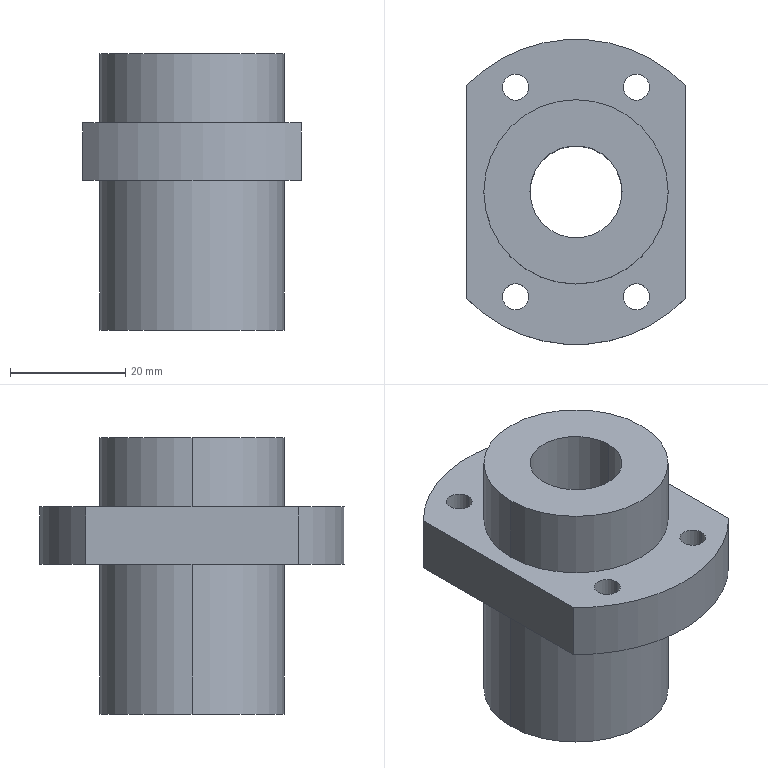Part | STEP file | Ball screw 4R16-16S2-DFSH-920-982-0.05(S)_HIWEI_default | 1 solid | 22 faces | box 38 x 53 x 48 mm | volume 38522 mm3 | cylinder 16 | plane 6 | commonest cylinder face diameters 4.5 x8 32 x4 16 x2 53 x2
STEP:
#1=CARTESIAN_POINT('',(-16.,0.,26.));
#2=VERTEX_POINT('',#1);
#3=CARTESIAN_POINT('',(16.,0.,26.));
#4=VERTEX_POINT('',#3);
#5=CARTESIAN_POINT('',(0.,0.,26.));
#6=DIRECTION('',(0.,0.,-1.));
#7=DIRECTION('',(-1.,0.,0.));
#8=AXIS2_PLACEMENT_3D('',#5,#6,#7);
#9=CIRCLE('',#8,16.);
#10=EDGE_CURVE('',#2,#4,#9,.T.);
#11=ORIENTED_EDGE('',*,*,#10,.T.);
#12=CARTESIAN_POINT('',(16.,0.,0.));
#13=VERTEX_POINT('',#12);
#14=CARTESIAN_POINT('',(16.,0.,48.));
#15=DIRECTION('',(0.,0.,-1.));
#16=VECTOR('',#15,1000.);
#17=LINE('',#14,#16);
#18=EDGE_CURVE('',#4,#13,#17,.T.);
#19=ORIENTED_EDGE('',*,*,#18,.T.);
#20=CARTESIAN_POINT('',(-16.,0.,0.));
#21=VERTEX_POINT('',#20);
#22=CARTESIAN_POINT('',(0.,0.,0.));
#23=DIRECTION('',(0.,0.,1.));
#24=DIRECTION('',(-1.,0.,0.));
#25=AXIS2_PLACEMENT_3D('',#22,#23,#24);
#26=CIRCLE('',#25,16.);
#27=EDGE_CURVE('',#13,#21,#26,.T.);
#28=ORIENTED_EDGE('',*,*,#27,.T.);
#29=CARTESIAN_POINT('',(-16.,0.,48.));
#30=DIRECTION('',(0.,0.,-1.));
#31=VECTOR('',#30,1000.);
#32=LINE('',#29,#31);
#33=EDGE_CURVE('',#2,#21,#32,.T.);
#34=ORIENTED_EDGE('',*,*,#33,.F.);
#35=EDGE_LOOP('',(#11,#19,#28,#34));
#36=FACE_OUTER_BOUND('',#35,.T.);
#37=CARTESIAN_POINT('',(0.,0.,48.));
#38=DIRECTION('',(0.,0.,-1.));
#39=DIRECTION('',(-1.,0.,0.));
#40=AXIS2_PLACEMENT_3D('',#37,#38,#39);
#41=CYLINDRICAL_SURFACE('',#40,16.);
#42=ADVANCED_FACE('',(#36),#41,.T.);
#43=CARTESIAN_POINT('',(8.,0.,48.));
#44=VERTEX_POINT('',#43);
#45=CARTESIAN_POINT('',(-8.,0.,48.));
#46=VERTEX_POINT('',#45);
#47=CARTESIAN_POINT('',(0.,0.,48.));
#48=DIRECTION('',(0.,0.,-1.));
#49=DIRECTION('',(-1.,0.,0.));
#50=AXIS2_PLACEMENT_3D('',#47,#48,#49);
#51=CIRCLE('',#50,8.);
#52=EDGE_CURVE('',#44,#46,#51,.T.);
#53=ORIENTED_EDGE('',*,*,#52,.F.);
#54=CARTESIAN_POINT('',(8.,0.,0.));
#55=VERTEX_POINT('',#54);
#56=CARTESIAN_POINT('',(8.,0.,160.));
#57=DIRECTION('',(0.,0.,-1.));
#58=VECTOR('',#57,1000.);
#59=LINE('',#56,#58);
#60=EDGE_CURVE('',#44,#55,#59,.T.);
#61=ORIENTED_EDGE('',*,*,#60,.T.);
#62=CARTESIAN_POINT('',(-8.,0.,0.));
#63=VERTEX_POINT('',#62);
#64=CARTESIAN_POINT('',(0.,0.,0.));
#65=DIRECTION('',(0.,0.,-1.));
#66=DIRECTION('',(-1.,0.,0.));
#67=AXIS2_PLACEMENT_3D('',#64,#65,#66);
#68=CIRCLE('',#67,8.);
#69=EDGE_CURVE('',#55,#63,#68,.T.);
#70=ORIENTED_EDGE('',*,*,#69,.T.);
#71=CARTESIAN_POINT('',(-8.,0.,160.));
#72=DIRECTION('',(0.,0.,-1.));
#73=VECTOR('',#72,1000.);
#74=LINE('',#71,#73);
#75=EDGE_CURVE('',#46,#63,#74,.T.);
#76=ORIENTED_EDGE('',*,*,#75,.F.);
#77=EDGE_LOOP('',(#53,#61,#70,#76));
#78=FACE_OUTER_BOUND('',#77,.T.);
#79=CARTESIAN_POINT('',(0.,0.,160.));
#80=DIRECTION('',(0.,0.,-1.));
#81=DIRECTION('',(-1.,0.,0.));
#82=AXIS2_PLACEMENT_3D('',#79,#80,#81);
#83=CYLINDRICAL_SURFACE('',#82,8.);
#84=ADVANCED_FACE('',(#78),#83,.F.);
#85=CARTESIAN_POINT('',(12.75,-18.187,26.));
#86=VERTEX_POINT('',#85);
#87=CARTESIAN_POINT('',(8.25,-18.187,26.));
#88=VERTEX_POINT('',#87);
#89=CARTESIAN_POINT('',(10.5,-18.187,26.));
#90=DIRECTION('',(0.,0.,-1.));
#91=DIRECTION('',(1.,0.,0.));
#92=AXIS2_PLACEMENT_3D('',#89,#90,#91);
#93=CIRCLE('',#92,2.25);
#94=EDGE_CURVE('',#86,#88,#93,.T.);
#95=ORIENTED_EDGE('',*,*,#94,.T.);
#96=CARTESIAN_POINT('',(8.25,-18.187,36.));
#97=VERTEX_POINT('',#96);
#98=CARTESIAN_POINT('',(8.25,-18.187,26.));
#99=DIRECTION('',(0.,0.,1.));
#100=VECTOR('',#99,1000.);
#101=LINE('',#98,#100);
#102=EDGE_CURVE('',#88,#97,#101,.T.);
#103=ORIENTED_EDGE('',*,*,#102,.T.);
#104=CARTESIAN_POINT('',(12.75,-18.187,36.));
#105=VERTEX_POINT('',#104);
#106=CARTESIAN_POINT('',(10.5,-18.187,36.));
#107=DIRECTION('',(0.,0.,-1.));
#108=DIRECTION('',(1.,0.,0.));
#109=AXIS2_PLACEMENT_3D('',#106,#107,#108);
#110=CIRCLE('',#109,2.25);
#111=EDGE_CURVE('',#105,#97,#110,.T.);
#112=ORIENTED_EDGE('',*,*,#111,.F.);
#113=CARTESIAN_POINT('',(12.75,-18.187,26.));
#114=DIRECTION('',(0.,0.,1.));
#115=VECTOR('',#114,1000.);
#116=LINE('',#113,#115);
#117=EDGE_CURVE('',#86,#105,#116,.T.);
#118=ORIENTED_EDGE('',*,*,#117,.F.);
#119=EDGE_LOOP('',(#95,#103,#112,#118));
#120=FACE_OUTER_BOUND('',#119,.T.);
#121=CARTESIAN_POINT('',(10.5,-18.187,26.));
#122=DIRECTION('',(0.,0.,1.));
#123=DIRECTION('',(1.,0.,0.));
#124=AXIS2_PLACEMENT_3D('',#121,#122,#123);
#125=CYLINDRICAL_SURFACE('',#124,2.25);
#126=ADVANCED_FACE('',(#120),#125,.F.);
#127=CARTESIAN_POINT('',(-8.25,18.187,26.));
#128=VERTEX_POINT('',#127);
#129=CARTESIAN_POINT('',(-12.75,18.187,26.));
#130=VERTEX_POINT('',#129);
#131=CARTESIAN_POINT('',(-10.5,18.187,26.));
#132=DIRECTION('',(0.,0.,-1.));
#133=DIRECTION('',(1.,0.,0.));
#134=AXIS2_PLACEMENT_3D('',#131,#132,#133);
#135=CIRCLE('',#134,2.25);
#136=EDGE_CURVE('',#128,#130,#135,.T.);
#137=ORIENTED_EDGE('',*,*,#136,.T.);
#138=CARTESIAN_POINT('',(-12.75,18.187,36.));
#139=VERTEX_POINT('',#138);
#140=CARTESIAN_POINT('',(-12.75,18.187,26.));
#141=DIRECTION('',(0.,0.,1.));
#142=VECTOR('',#141,1000.);
#143=LINE('',#140,#142);
#144=EDGE_CURVE('',#130,#139,#143,.T.);
#145=ORIENTED_EDGE('',*,*,#144,.T.);
#146=CARTESIAN_POINT('',(-8.25,18.187,36.));
#147=VERTEX_POINT('',#146);
#148=CARTESIAN_POINT('',(-10.5,18.187,36.));
#149=DIRECTION('',(0.,0.,-1.));
#150=DIRECTION('',(1.,0.,0.));
#151=AXIS2_PLACEMENT_3D('',#148,#149,#150);
#152=CIRCLE('',#151,2.25);
#153=EDGE_CURVE('',#147,#139,#152,.T.);
#154=ORIENTED_EDGE('',*,*,#153,.F.);
#155=CARTESIAN_POINT('',(-8.25,18.187,26.));
#156=DIRECTION('',(0.,0.,1.));
#157=VECTOR('',#156,1000.);
#158=LINE('',#155,#157);
#159=EDGE_CURVE('',#128,#147,#158,.T.);
#160=ORIENTED_EDGE('',*,*,#159,.F.);
#161=EDGE_LOOP('',(#137,#145,#154,#160));
#162=FACE_OUTER_BOUND('',#161,.T.);
#163=CARTESIAN_POINT('',(-10.5,18.187,26.));
#164=DIRECTION('',(0.,0.,1.));
#165=DIRECTION('',(1.,0.,0.));
#166=AXIS2_PLACEMENT_3D('',#163,#164,#165);
#167=CYLINDRICAL_SURFACE('',#166,2.25);
#168=ADVANCED_FACE('',(#162),#167,.F.);
#169=CARTESIAN_POINT('',(12.75,18.187,26.));
#170=VERTEX_POINT('',#169);
#171=CARTESIAN_POINT('',(8.25,18.187,26.));
#172=VERTEX_POINT('',#171);
#173=CARTESIAN_POINT('',(10.5,18.187,26.));
#174=DIRECTION('',(0.,0.,-1.));
#175=DIRECTION('',(1.,0.,0.));
#176=AXIS2_PLACEMENT_3D('',#173,#174,#175);
#177=CIRCLE('',#176,2.25);
#178=EDGE_CURVE('',#170,#172,#177,.T.);
#179=ORIENTED_EDGE('',*,*,#178,.T.);
#180=CARTESIAN_POINT('',(8.25,18.187,36.));
#181=VERTEX_POINT('',#180);
#182=CARTESIAN_POINT('',(8.25,18.187,26.));
#183=DIRECTION('',(0.,0.,1.));
#184=VECTOR('',#183,1000.);
#185=LINE('',#182,#184);
#186=EDGE_CURVE('',#172,#181,#185,.T.);
#187=ORIENTED_EDGE('',*,*,#186,.T.);
#188=CARTESIAN_POINT('',(12.75,18.187,36.));
#189=VERTEX_POINT('',#188);
#190=CARTESIAN_POINT('',(10.5,18.187,36.));
#191=DIRECTION('',(0.,0.,-1.));
#192=DIRECTION('',(1.,0.,0.));
#193=AXIS2_PLACEMENT_3D('',#190,#191,#192);
#194=CIRCLE('',#193,2.25);
#195=EDGE_CURVE('',#189,#181,#194,.T.);
#196=ORIENTED_EDGE('',*,*,#195,.F.);
#197=CARTESIAN_POINT('',(12.75,18.187,26.));
#198=DIRECTION('',(0.,0.,1.));
#199=VECTOR('',#198,1000.);
#200=LINE('',#197,#199);
#201=EDGE_CURVE('',#170,#189,#200,.T.);
#202=ORIENTED_EDGE('',*,*,#201,.F.);
#203=EDGE_LOOP('',(#179,#187,#196,#202));
#204=FACE_OUTER_BOUND('',#203,.T.);
#205=CARTESIAN_POINT('',(10.5,18.187,26.));
#206=DIRECTION('',(0.,0.,1.));
#207=DIRECTION('',(1.,0.,0.));
#208=AXIS2_PLACEMENT_3D('',#205,#206,#207);
#209=CYLINDRICAL_SURFACE('',#208,2.25);
#210=ADVANCED_FACE('',(#204),#209,.F.);
#211=CARTESIAN_POINT('',(-8.25,-18.187,26.));
#212=VERTEX_POINT('',#211);
#213=CARTESIAN_POINT('',(-12.75,-18.187,26.));
#214=VERTEX_POINT('',#213);
#215=CARTESIAN_POINT('',(-10.5,-18.187,26.));
#216=DIRECTION('',(0.,0.,-1.));
#217=DIRECTION('',(1.,0.,0.));
#218=AXIS2_PLACEMENT_3D('',#215,#216,#217);
#219=CIRCLE('',#218,2.25);
#220=EDGE_CURVE('',#212,#214,#219,.T.);
#221=ORIENTED_EDGE('',*,*,#220,.T.);
#222=CARTESIAN_POINT('',(-12.75,-18.187,36.));
#223=VERTEX_POINT('',#222);
#224=CARTESIAN_POINT('',(-12.75,-18.187,26.));
#225=DIRECTION('',(0.,0.,1.));
#226=VECTOR('',#225,1000.);
#227=LINE('',#224,#226);
#228=EDGE_CURVE('',#214,#223,#227,.T.);
#229=ORIENTED_EDGE('',*,*,#228,.T.);
#230=CARTESIAN_POINT('',(-8.25,-18.187,36.));
#231=VERTEX_POINT('',#230);
#232=CARTESIAN_POINT('',(-10.5,-18.187,36.));
#233=DIRECTION('',(0.,0.,-1.));
#234=DIRECTION('',(1.,0.,0.));
#235=AXIS2_PLACEMENT_3D('',#232,#233,#234);
#236=CIRCLE('',#235,2.25);
#237=EDGE_CURVE('',#231,#223,#236,.T.);
#238=ORIENTED_EDGE('',*,*,#237,.F.);
#239=CARTESIAN_POINT('',(-8.25,-18.187,26.));
#240=DIRECTION('',(0.,0.,1.));
#241=VECTOR('',#240,1000.);
#242=LINE('',#239,#241);
#243=EDGE_CURVE('',#212,#231,#242,.T.);
#244=ORIENTED_EDGE('',*,*,#243,.F.);
#245=EDGE_LOOP('',(#221,#229,#238,#244));
#246=FACE_OUTER_BOUND('',#245,.T.);
#247=CARTESIAN_POINT('',(-10.5,-18.187,26.));
#248=DIRECTION('',(0.,0.,1.));
#249=DIRECTION('',(1.,0.,0.));
#250=AXIS2_PLACEMENT_3D('',#247,#248,#249);
#251=CYLINDRICAL_SURFACE('',#250,2.25);
#252=ADVANCED_FACE('',(#246),#251,.F.);
#253=CARTESIAN_POINT('',(16.,0.,48.));
#254=VERTEX_POINT('',#253);
#255=CARTESIAN_POINT('',(-16.,0.,48.));
#256=VERTEX_POINT('',#255);
#257=CARTESIAN_POINT('',(0.,0.,48.));
#258=DIRECTION('',(0.,0.,1.));
#259=DIRECTION('',(-1.,0.,0.));
#260=AXIS2_PLACEMENT_3D('',#257,#258,#259);
#261=CIRCLE('',#260,16.);
#262=EDGE_CURVE('',#254,#256,#261,.T.);
#263=ORIENTED_EDGE('',*,*,#262,.F.);
#264=CARTESIAN_POINT('',(16.,0.,36.));
#265=VERTEX_POINT('',#264);
#266=CARTESIAN_POINT('',(16.,0.,48.));
#267=DIRECTION('',(0.,0.,-1.));
#268=VECTOR('',#267,1000.);
#269=LINE('',#266,#268);
#270=EDGE_CURVE('',#254,#265,#269,.T.);
#271=ORIENTED_EDGE('',*,*,#270,.T.);
#272=CARTESIAN_POINT('',(-16.,0.,36.));
#273=VERTEX_POINT('',#272);
#274=CARTESIAN_POINT('',(0.,0.,36.));
#275=DIRECTION('',(0.,0.,-1.));
#276=DIRECTION('',(-1.,0.,0.));
#277=AXIS2_PLACEMENT_3D('',#274,#275,#276);
#278=CIRCLE('',#277,16.);
#279=EDGE_CURVE('',#273,#265,#278,.T.);
#280=ORIENTED_EDGE('',*,*,#279,.F.);
#281=CARTESIAN_POINT('',(-16.,0.,48.));
#282=DIRECTION('',(0.,0.,-1.));
#283=VECTOR('',#282,1000.);
#284=LINE('',#281,#283);
#285=EDGE_CURVE('',#256,#273,#284,.T.);
#286=ORIENTED_EDGE('',*,*,#285,.F.);
#287=EDGE_LOOP('',(#263,#271,#280,#286));
#288=FACE_OUTER_BOUND('',#287,.T.);
#289=CARTESIAN_POINT('',(0.,0.,48.));
#290=DIRECTION('',(0.,0.,-1.));
#291=DIRECTION('',(-1.,0.,0.));
#292=AXIS2_PLACEMENT_3D('',#289,#290,#291);
#293=CYLINDRICAL_SURFACE('',#292,16.);
#294=ADVANCED_FACE('',(#288),#293,.T.);
#295=ORIENTED_EDGE('',*,*,#18,.F.);
#296=CARTESIAN_POINT('',(0.,0.,26.));
#297=DIRECTION('',(0.,0.,-1.));
#298=DIRECTION('',(-1.,0.,0.));
#299=AXIS2_PLACEMENT_3D('',#296,#297,#298);
#300=CIRCLE('',#299,16.);
#301=EDGE_CURVE('',#4,#2,#300,.T.);
#302=ORIENTED_EDGE('',*,*,#301,.T.);
#303=ORIENTED_EDGE('',*,*,#33,.T.);
#304=CARTESIAN_POINT('',(0.,0.,0.));
#305=DIRECTION('',(0.,0.,1.));
#306=DIRECTION('',(-1.,0.,0.));
#307=AXIS2_PLACEMENT_3D('',#304,#305,#306);
#308=CIRCLE('',#307,16.);
#309=EDGE_CURVE('',#21,#13,#308,.T.);
#310=ORIENTED_EDGE('',*,*,#309,.T.);
#311=EDGE_LOOP('',(#295,#302,#303,#310));
#312=FACE_OUTER_BOUND('',#311,.T.);
#313=CARTESIAN_POINT('',(0.,0.,48.));
#314=DIRECTION('',(0.,0.,-1.));
#315=DIRECTION('',(-1.,0.,0.));
#316=AXIS2_PLACEMENT_3D('',#313,#314,#315);
#317=CYLINDRICAL_SURFACE('',#316,16.);
#318=ADVANCED_FACE('',(#312),#317,.T.);
#319=ORIENTED_EDGE('',*,*,#309,.F.);
#320=ORIENTED_EDGE('',*,*,#27,.F.);
#321=EDGE_LOOP('',(#319,#320));
#322=FACE_OUTER_BOUND('',#321,.T.);
#323=CARTESIAN_POINT('',(0.,0.,0.));
#324=DIRECTION('',(0.,0.,-1.));
#325=DIRECTION('',(-1.,0.,0.));
#326=AXIS2_PLACEMENT_3D('',#323,#324,#325);
#327=CIRCLE('',#326,8.);
#328=EDGE_CURVE('',#63,#55,#327,.T.);
#329=ORIENTED_EDGE('',*,*,#328,.F.);
#330=ORIENTED_EDGE('',*,*,#69,.F.);
#331=EDGE_LOOP('',(#329,#330));
#332=FACE_BOUND('',#331,.T.);
#333=CARTESIAN_POINT('',(0.,0.,0.));
#334=DIRECTION('',(0.,0.,1.));
#335=DIRECTION('',(1.,0.,0.));
#336=AXIS2_PLACEMENT_3D('',#333,#334,#335);
#337=PLANE('',#336);
#338=ADVANCED_FACE('',(#322,#332),#337,.F.);
#339=ORIENTED_EDGE('',*,*,#94,.F.);
#340=CARTESIAN_POINT('',(10.5,-18.187,26.));
#341=DIRECTION('',(0.,0.,-1.));
#342=DIRECTION('',(1.,0.,0.));
#343=AXIS2_PLACEMENT_3D('',#340,#341,#342);
#344=CIRCLE('',#343,2.25);
#345=EDGE_CURVE('',#88,#86,#344,.T.);
#346=ORIENTED_EDGE('',*,*,#345,.F.);
#347=EDGE_LOOP('',(#339,#346));
#348=FACE_BOUND('',#347,.T.);
#349=ORIENTED_EDGE('',*,*,#10,.F.);
#350=ORIENTED_EDGE('',*,*,#301,.F.);
#351=EDGE_LOOP('',(#349,#350));
#352=FACE_BOUND('',#351,.T.);
#353=CARTESIAN_POINT('',(19.,-18.473,26.));
#354=VERTEX_POINT('',#353);
#355=CARTESIAN_POINT('',(19.,18.473,26.));
#356=VERTEX_POINT('',#355);
#357=CARTESIAN_POINT('',(19.,0.,26.));
#358=DIRECTION('',(0.,1.,0.));
#359=VECTOR('',#358,1000.);
#360=LINE('',#357,#359);
#361=EDGE_CURVE('',#354,#356,#360,.T.);
#362=ORIENTED_EDGE('',*,*,#361,.F.);
#363=CARTESIAN_POINT('',(-19.,-18.473,26.));
#364=VERTEX_POINT('',#363);
#365=CARTESIAN_POINT('',(0.,0.,26.));
#366=DIRECTION('',(0.,0.,1.));
#367=DIRECTION('',(-1.,0.,0.));
#368=AXIS2_PLACEMENT_3D('',#365,#366,#367);
#369=CIRCLE('',#368,26.5);
#370=EDGE_CURVE('',#364,#354,#369,.T.);
#371=ORIENTED_EDGE('',*,*,#370,.F.);
#372=CARTESIAN_POINT('',(-19.,18.473,26.));
#373=VERTEX_POINT('',#372);
#374=CARTESIAN_POINT('',(-19.,0.,26.));
#375=DIRECTION('',(0.,-1.,0.));
#376=VECTOR('',#375,1000.);
#377=LINE('',#374,#376);
#378=EDGE_CURVE('',#373,#364,#377,.T.);
#379=ORIENTED_EDGE('',*,*,#378,.F.);
#380=CARTESIAN_POINT('',(0.,0.,26.));
#381=DIRECTION('',(0.,0.,1.));
#382=DIRECTION('',(-1.,0.,0.));
#383=AXIS2_PLACEMENT_3D('',#380,#381,#382);
#384=CIRCLE('',#383,26.5);
#385=EDGE_CURVE('',#356,#373,#384,.T.);
#386=ORIENTED_EDGE('',*,*,#385,.F.);
#387=EDGE_LOOP('',(#362,#371,#379,#386));
#388=FACE_OUTER_BOUND('',#387,.T.);
#389=ORIENTED_EDGE('',*,*,#136,.F.);
#390=CARTESIAN_POINT('',(-10.5,18.187,26.));
#391=DIRECTION('',(0.,0.,-1.));
#392=DIRECTION('',(1.,0.,0.));
#393=AXIS2_PLACEMENT_3D('',#390,#391,#392);
#394=CIRCLE('',#393,2.25);
#395=EDGE_CURVE('',#130,#128,#394,.T.);
#396=ORIENTED_EDGE('',*,*,#395,.F.);
#397=EDGE_LOOP('',(#389,#396));
#398=FACE_BOUND('',#397,.T.);
#399=ORIENTED_EDGE('',*,*,#178,.F.);
#400=CARTESIAN_POINT('',(10.5,18.187,26.));
#401=DIRECTION('',(0.,0.,-1.));
#402=DIRECTION('',(1.,0.,0.));
#403=AXIS2_PLACEMENT_3D('',#400,#401,#402);
#404=CIRCLE('',#403,2.25);
#405=EDGE_CURVE('',#172,#170,#404,.T.);
#406=ORIENTED_EDGE('',*,*,#405,.F.);
#407=EDGE_LOOP('',(#399,#406));
#408=FACE_BOUND('',#407,.T.);
#409=ORIENTED_EDGE('',*,*,#220,.F.);
#410=CARTESIAN_POINT('',(-10.5,-18.187,26.));
#411=DIRECTION('',(0.,0.,-1.));
#412=DIRECTION('',(1.,0.,0.));
#413=AXIS2_PLACEMENT_3D('',#410,#411,#412);
#414=CIRCLE('',#413,2.25);
#415=EDGE_CURVE('',#214,#212,#414,.T.);
#416=ORIENTED_EDGE('',*,*,#415,.F.);
#417=EDGE_LOOP('',(#409,#416));
#418=FACE_BOUND('',#417,.T.);
#419=CARTESIAN_POINT('',(0.,0.,26.));
#420=DIRECTION('',(0.,0.,1.));
#421=DIRECTION('',(1.,0.,0.));
#422=AXIS2_PLACEMENT_3D('',#419,#420,#421);
#423=PLANE('',#422);
#424=ADVANCED_FACE('',(#348,#352,#388,#398,#408,#418),#423,.F.);
#425=ORIENTED_EDGE('',*,*,#60,.F.);
#426=CARTESIAN_POINT('',(0.,0.,48.));
#427=DIRECTION('',(0.,0.,-1.));
#428=DIRECTION('',(-1.,0.,0.));
#429=AXIS2_PLACEMENT_3D('',#426,#427,#428);
#430=CIRCLE('',#429,8.);
#431=EDGE_CURVE('',#46,#44,#430,.T.);
#432=ORIENTED_EDGE('',*,*,#431,.F.);
#433=ORIENTED_EDGE('',*,*,#75,.T.);
#434=ORIENTED_EDGE('',*,*,#328,.T.);
#435=EDGE_LOOP('',(#425,#432,#433,#434));
#436=FACE_OUTER_BOUND('',#435,.T.);
#437=CARTESIAN_POINT('',(0.,0.,160.));
#438=DIRECTION('',(0.,0.,-1.));
#439=DIRECTION('',(-1.,0.,0.));
#440=AXIS2_PLACEMENT_3D('',#437,#438,#439);
#441=CYLINDRICAL_SURFACE('',#440,8.);
#442=ADVANCED_FACE('',(#436),#441,.F.);
#443=ORIENTED_EDGE('',*,*,#102,.F.);
#444=ORIENTED_EDGE('',*,*,#345,.T.);
#445=ORIENTED_EDGE('',*,*,#117,.T.);
#446=CARTESIAN_POINT('',(10.5,-18.187,36.));
#447=DIRECTION('',(0.,0.,-1.));
#448=DIRECTION('',(1.,0.,0.));
#449=AXIS2_PLACEMENT_3D('',#446,#447,#448);
#450=CIRCLE('',#449,2.25);
#451=EDGE_CURVE('',#97,#105,#450,.T.);
#452=ORIENTED_EDGE('',*,*,#451,.F.);
#453=EDGE_LOOP('',(#443,#444,#445,#452));
#454=FACE_OUTER_BOUND('',#453,.T.);
#455=CARTESIAN_POINT('',(10.5,-18.187,26.));
#456=DIRECTION('',(0.,0.,1.));
#457=DIRECTION('',(1.,0.,0.));
#458=AXIS2_PLACEMENT_3D('',#455,#456,#457);
#459=CYLINDRICAL_SURFACE('',#458,2.25);
#460=ADVANCED_FACE('',(#454),#459,.F.);
#461=ORIENTED_EDGE('',*,*,#385,.T.);
#462=CARTESIAN_POINT('',(-19.,18.473,36.));
#463=VERTEX_POINT('',#462);
#464=CARTESIAN_POINT('',(-19.,18.473,36.));
#465=DIRECTION('',(0.,0.,1.));
#466=VECTOR('',#465,1000.);
#467=LINE('',#464,#466);
#468=EDGE_CURVE('',#373,#463,#467,.T.);
#469=ORIENTED_EDGE('',*,*,#468,.T.);
#470=CARTESIAN_POINT('',(19.,18.473,36.));
#471=VERTEX_POINT('',#470);
#472=CARTESIAN_POINT('',(0.,0.,36.));
#473=DIRECTION('',(0.,0.,-1.));
#474=DIRECTION('',(-1.,0.,0.));
#475=AXIS2_PLACEMENT_3D('',#472,#473,#474);
#476=CIRCLE('',#475,26.5);
#477=EDGE_CURVE('',#463,#471,#476,.T.);
#478=ORIENTED_EDGE('',*,*,#477,.T.);
#479=CARTESIAN_POINT('',(19.,18.473,36.));
#480=DIRECTION('',(0.,0.,-1.));
#481=VECTOR('',#480,1000.);
#482=LINE('',#479,#481);
#483=EDGE_CURVE('',#471,#356,#482,.T.);
#484=ORIENTED_EDGE('',*,*,#483,.T.);
#485=EDGE_LOOP('',(#461,#469,#478,#484));
#486=FACE_OUTER_BOUND('',#485,.T.);
#487=CARTESIAN_POINT('',(0.,0.,36.));
#488=DIRECTION('',(0.,0.,-1.));
#489=DIRECTION('',(-1.,0.,0.));
#490=AXIS2_PLACEMENT_3D('',#487,#488,#489);
#491=CYLINDRICAL_SURFACE('',#490,26.5);
#492=ADVANCED_FACE('',(#486),#491,.T.);
#493=CARTESIAN_POINT('',(19.,-18.473,36.));
#494=VERTEX_POINT('',#493);
#495=CARTESIAN_POINT('',(19.,-18.473,26.));
#496=DIRECTION('',(0.,0.,1.));
#497=VECTOR('',#496,1000.);
#498=LINE('',#495,#497);
#499=EDGE_CURVE('',#354,#494,#498,.T.);
#500=ORIENTED_EDGE('',*,*,#499,.F.);
#501=ORIENTED_EDGE('',*,*,#361,.T.);
#502=ORIENTED_EDGE('',*,*,#483,.F.);
#503=CARTESIAN_POINT('',(19.,21.909,36.));
#504=DIRECTION('',(0.,1.,0.));
#505=VECTOR('',#504,1000.);
#506=LINE('',#503,#505);
#507=EDGE_CURVE('',#494,#471,#506,.T.);
#508=ORIENTED_EDGE('',*,*,#507,.F.);
#509=EDGE_LOOP('',(#500,#501,#502,#508));
#510=FACE_OUTER_BOUND('',#509,.T.);
#511=CARTESIAN_POINT('',(19.,21.909,26.));
#512=DIRECTION('',(-1.,0.,0.));
#513=DIRECTION('',(0.,0.,1.));
#514=AXIS2_PLACEMENT_3D('',#511,#512,#513);
#515=PLANE('',#514);
#516=ADVANCED_FACE('',(#510),#515,.F.);
#517=CARTESIAN_POINT('',(-19.,-18.473,36.));
#518=VERTEX_POINT('',#517);
#519=CARTESIAN_POINT('',(0.,0.,36.));
#520=DIRECTION('',(0.,0.,-1.));
#521=DIRECTION('',(-1.,0.,0.));
#522=AXIS2_PLACEMENT_3D('',#519,#520,#521);
#523=CIRCLE('',#522,26.5);
#524=EDGE_CURVE('',#494,#518,#523,.T.);
#525=ORIENTED_EDGE('',*,*,#524,.T.);
#526=CARTESIAN_POINT('',(-19.,-18.473,36.));
#527=DIRECTION('',(0.,0.,-1.));
#528=VECTOR('',#527,1000.);
#529=LINE('',#526,#528);
#530=EDGE_CURVE('',#518,#364,#529,.T.);
#531=ORIENTED_EDGE('',*,*,#530,.T.);
#532=ORIENTED_EDGE('',*,*,#370,.T.);
#533=ORIENTED_EDGE('',*,*,#499,.T.);
#534=EDGE_LOOP('',(#525,#531,#532,#533));
#535=FACE_OUTER_BOUND('',#534,.T.);
#536=CARTESIAN_POINT('',(0.,0.,36.));
#537=DIRECTION('',(0.,0.,-1.));
#538=DIRECTION('',(-1.,0.,0.));
#539=AXIS2_PLACEMENT_3D('',#536,#537,#538);
#540=CYLINDRICAL_SURFACE('',#539,26.5);
#541=ADVANCED_FACE('',(#535),#540,.T.);
#542=ORIENTED_EDGE('',*,*,#468,.F.);
#543=ORIENTED_EDGE('',*,*,#378,.T.);
#544=ORIENTED_EDGE('',*,*,#530,.F.);
#545=CARTESIAN_POINT('',(-19.,21.909,36.));
#546=DIRECTION('',(0.,-1.,0.));
#547=VECTOR('',#546,1000.);
#548=LINE('',#545,#547);
#549=EDGE_CURVE('',#463,#518,#548,.T.);
#550=ORIENTED_EDGE('',*,*,#549,.F.);
#551=EDGE_LOOP('',(#542,#543,#544,#550));
#552=FACE_OUTER_BOUND('',#551,.T.);
#553=CARTESIAN_POINT('',(-19.,21.909,26.));
#554=DIRECTION('',(1.,0.,0.));
#555=DIRECTION('',(0.,0.,-1.));
#556=AXIS2_PLACEMENT_3D('',#553,#554,#555);
#557=PLANE('',#556);
#558=ADVANCED_FACE('',(#552),#557,.F.);
#559=ORIENTED_EDGE('',*,*,#144,.F.);
#560=ORIENTED_EDGE('',*,*,#395,.T.);
#561=ORIENTED_EDGE('',*,*,#159,.T.);
#562=CARTESIAN_POINT('',(-10.5,18.187,36.));
#563=DIRECTION('',(0.,0.,-1.));
#564=DIRECTION('',(1.,0.,0.));
#565=AXIS2_PLACEMENT_3D('',#562,#563,#564);
#566=CIRCLE('',#565,2.25);
#567=EDGE_CURVE('',#139,#147,#566,.T.);
#568=ORIENTED_EDGE('',*,*,#567,.F.);
#569=EDGE_LOOP('',(#559,#560,#561,#568));
#570=FACE_OUTER_BOUND('',#569,.T.);
#571=CARTESIAN_POINT('',(-10.5,18.187,26.));
#572=DIRECTION('',(0.,0.,1.));
#573=DIRECTION('',(1.,0.,0.));
#574=AXIS2_PLACEMENT_3D('',#571,#572,#573);
#575=CYLINDRICAL_SURFACE('',#574,2.25);
#576=ADVANCED_FACE('',(#570),#575,.F.);
#577=ORIENTED_EDGE('',*,*,#186,.F.);
#578=ORIENTED_EDGE('',*,*,#405,.T.);
#579=ORIENTED_EDGE('',*,*,#201,.T.);
#580=CARTESIAN_POINT('',(10.5,18.187,36.));
#581=DIRECTION('',(0.,0.,-1.));
#582=DIRECTION('',(1.,0.,0.));
#583=AXIS2_PLACEMENT_3D('',#580,#581,#582);
#584=CIRCLE('',#583,2.25);
#585=EDGE_CURVE('',#181,#189,#584,.T.);
#586=ORIENTED_EDGE('',*,*,#585,.F.);
#587=EDGE_LOOP('',(#577,#578,#579,#586));
#588=FACE_OUTER_BOUND('',#587,.T.);
#589=CARTESIAN_POINT('',(10.5,18.187,26.));
#590=DIRECTION('',(0.,0.,1.));
#591=DIRECTION('',(1.,0.,0.));
#592=AXIS2_PLACEMENT_3D('',#589,#590,#591);
#593=CYLINDRICAL_SURFACE('',#592,2.25);
#594=ADVANCED_FACE('',(#588),#593,.F.);
#595=ORIENTED_EDGE('',*,*,#228,.F.);
#596=ORIENTED_EDGE('',*,*,#415,.T.);
#597=ORIENTED_EDGE('',*,*,#243,.T.);
#598=CARTESIAN_POINT('',(-10.5,-18.187,36.));
#599=DIRECTION('',(0.,0.,-1.));
#600=DIRECTION('',(1.,0.,0.));
#601=AXIS2_PLACEMENT_3D('',#598,#599,#600);
#602=CIRCLE('',#601,2.25);
#603=EDGE_CURVE('',#223,#231,#602,.T.);
#604=ORIENTED_EDGE('',*,*,#603,.F.);
#605=EDGE_LOOP('',(#595,#596,#597,#604));
#606=FACE_OUTER_BOUND('',#605,.T.);
#607=CARTESIAN_POINT('',(-10.5,-18.187,26.));
#608=DIRECTION('',(0.,0.,1.));
#609=DIRECTION('',(1.,0.,0.));
#610=AXIS2_PLACEMENT_3D('',#607,#608,#609);
#611=CYLINDRICAL_SURFACE('',#610,2.25);
#612=ADVANCED_FACE('',(#606),#611,.F.);
#613=CARTESIAN_POINT('',(0.,0.,48.));
#614=DIRECTION('',(0.,0.,1.));
#615=DIRECTION('',(-1.,0.,0.));
#616=AXIS2_PLACEMENT_3D('',#613,#614,#615);
#617=CIRCLE('',#616,16.);
#618=EDGE_CURVE('',#256,#254,#617,.T.);
#619=ORIENTED_EDGE('',*,*,#618,.T.);
#620=ORIENTED_EDGE('',*,*,#262,.T.);
#621=EDGE_LOOP('',(#619,#620));
#622=FACE_OUTER_BOUND('',#621,.T.);
#623=ORIENTED_EDGE('',*,*,#431,.T.);
#624=ORIENTED_EDGE('',*,*,#52,.T.);
#625=EDGE_LOOP('',(#623,#624));
#626=FACE_BOUND('',#625,.T.);
#627=CARTESIAN_POINT('',(0.,0.,48.));
#628=DIRECTION('',(0.,0.,1.));
#629=DIRECTION('',(1.,0.,0.));
#630=AXIS2_PLACEMENT_3D('',#627,#628,#629);
#631=PLANE('',#630);
#632=ADVANCED_FACE('',(#622,#626),#631,.T.);
#633=ORIENTED_EDGE('',*,*,#111,.T.);
#634=ORIENTED_EDGE('',*,*,#451,.T.);
#635=EDGE_LOOP('',(#633,#634));
#636=FACE_BOUND('',#635,.T.);
#637=ORIENTED_EDGE('',*,*,#279,.T.);
#638=CARTESIAN_POINT('',(0.,0.,36.));
#639=DIRECTION('',(0.,0.,-1.));
#640=DIRECTION('',(-1.,0.,0.));
#641=AXIS2_PLACEMENT_3D('',#638,#639,#640);
#642=CIRCLE('',#641,16.);
#643=EDGE_CURVE('',#265,#273,#642,.T.);
#644=ORIENTED_EDGE('',*,*,#643,.T.);
#645=EDGE_LOOP('',(#637,#644));
#646=FACE_BOUND('',#645,.T.);
#647=ORIENTED_EDGE('',*,*,#153,.T.);
#648=ORIENTED_EDGE('',*,*,#567,.T.);
#649=EDGE_LOOP('',(#647,#648));
#650=FACE_BOUND('',#649,.T.);
#651=ORIENTED_EDGE('',*,*,#195,.T.);
#652=ORIENTED_EDGE('',*,*,#585,.T.);
#653=EDGE_LOOP('',(#651,#652));
#654=FACE_BOUND('',#653,.T.);
#655=ORIENTED_EDGE('',*,*,#237,.T.);
#656=ORIENTED_EDGE('',*,*,#603,.T.);
#657=EDGE_LOOP('',(#655,#656));
#658=FACE_BOUND('',#657,.T.);
#659=ORIENTED_EDGE('',*,*,#549,.T.);
#660=ORIENTED_EDGE('',*,*,#524,.F.);
#661=ORIENTED_EDGE('',*,*,#507,.T.);
#662=ORIENTED_EDGE('',*,*,#477,.F.);
#663=EDGE_LOOP('',(#659,#660,#661,#662));
#664=FACE_OUTER_BOUND('',#663,.T.);
#665=CARTESIAN_POINT('',(0.,0.,36.));
#666=DIRECTION('',(0.,0.,1.));
#667=DIRECTION('',(1.,0.,0.));
#668=AXIS2_PLACEMENT_3D('',#665,#666,#667);
#669=PLANE('',#668);
#670=ADVANCED_FACE('',(#636,#646,#650,#654,#658,#664),#669,.T.);
#671=ORIENTED_EDGE('',*,*,#270,.F.);
#672=ORIENTED_EDGE('',*,*,#618,.F.);
#673=ORIENTED_EDGE('',*,*,#285,.T.);
#674=ORIENTED_EDGE('',*,*,#643,.F.);
#675=EDGE_LOOP('',(#671,#672,#673,#674));
#676=FACE_OUTER_BOUND('',#675,.T.);
#677=CARTESIAN_POINT('',(0.,0.,48.));
#678=DIRECTION('',(0.,0.,-1.));
#679=DIRECTION('',(-1.,0.,0.));
#680=AXIS2_PLACEMENT_3D('',#677,#678,#679);
#681=CYLINDRICAL_SURFACE('',#680,16.);
#682=ADVANCED_FACE('',(#676),#681,.T.);
#683=CLOSED_SHELL('',(#42,#84,#126,#168,#210,#252,#294,#318,#338,#424,#442,#460,#492,#516,#541,#558,#576,#594,#612,#632,#670,#682));
#684=MANIFOLD_SOLID_BREP('',#683);
#685=CARTESIAN_POINT('',(0.,0.,0.));
#686=DIRECTION('',(0.,0.,1.));
#687=DIRECTION('',(1.,0.,0.));
#688=AXIS2_PLACEMENT_3D('',#685,#686,#687);
#689=(LENGTH_UNIT()NAMED_UNIT(*)SI_UNIT(.MILLI.,.METRE.));
#690=UNCERTAINTY_MEASURE_WITH_UNIT(LENGTH_MEASURE(0.00001),#689,'','');
#691=(NAMED_UNIT(*)PLANE_ANGLE_UNIT()SI_UNIT($,.RADIAN.));
#692=(NAMED_UNIT(*)SI_UNIT($,.STERADIAN.)SOLID_ANGLE_UNIT());
#693=(GEOMETRIC_REPRESENTATION_CONTEXT(3)GLOBAL_UNCERTAINTY_ASSIGNED_CONTEXT((#690))GLOBAL_UNIT_ASSIGNED_CONTEXT((#689,#691,#692))REPRESENTATION_CONTEXT('',''));
#694=ADVANCED_BREP_SHAPE_REPRESENTATION('',(#684,#688),#693);